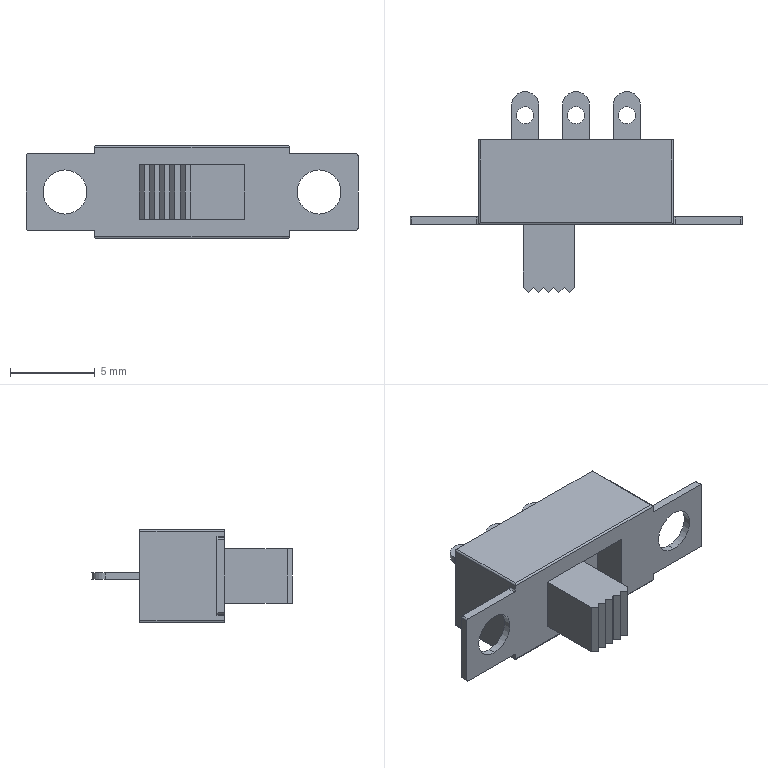Part | SolidWorks | features BaseBody 1 | 1 solid | 71 faces | box 19.6 x 11.85 x 5.5 mm | volume 348.463 mm3 | plane 44 | cylinder 27 | commonest cylinder face diameters 0.2 x14 1 x6 2.6 x4 1.6 x3